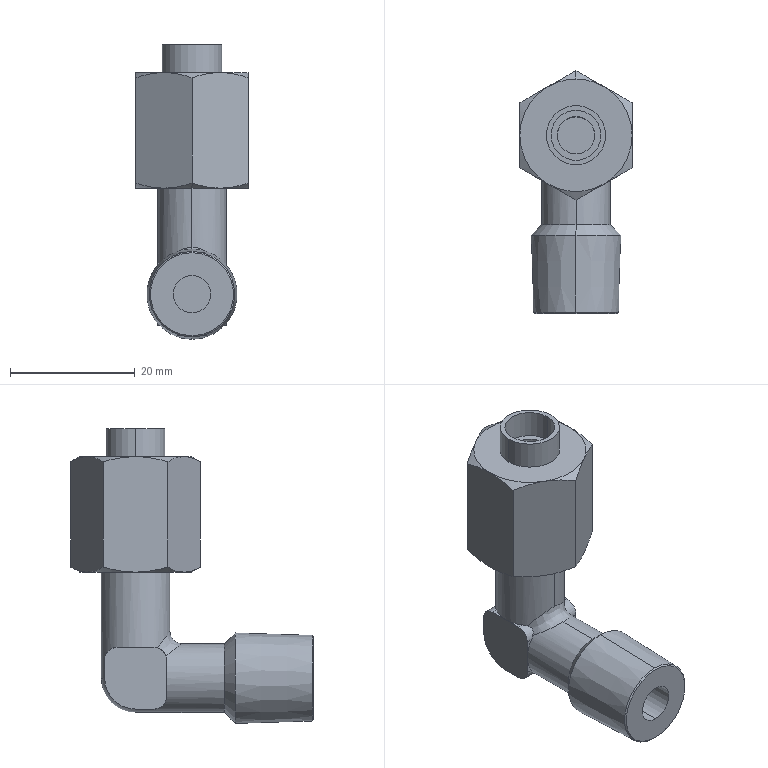Part | SolidWorks | features Boss 4, Fillet 2, RevCut 2, Revolution 2, Chamfer 1, ICE 1, Sweep 1 | 1 solid | 69 faces | box 18 x 38.892 x 47.244 mm | volume 8990 mm3 | plane 27 | cone 20 | cylinder 20 | sphere 1 | spline 1 | commonest cylinder face diameters 4 x6 6 x4 11 x4 8 x2 9.5 x2 9.9 x2